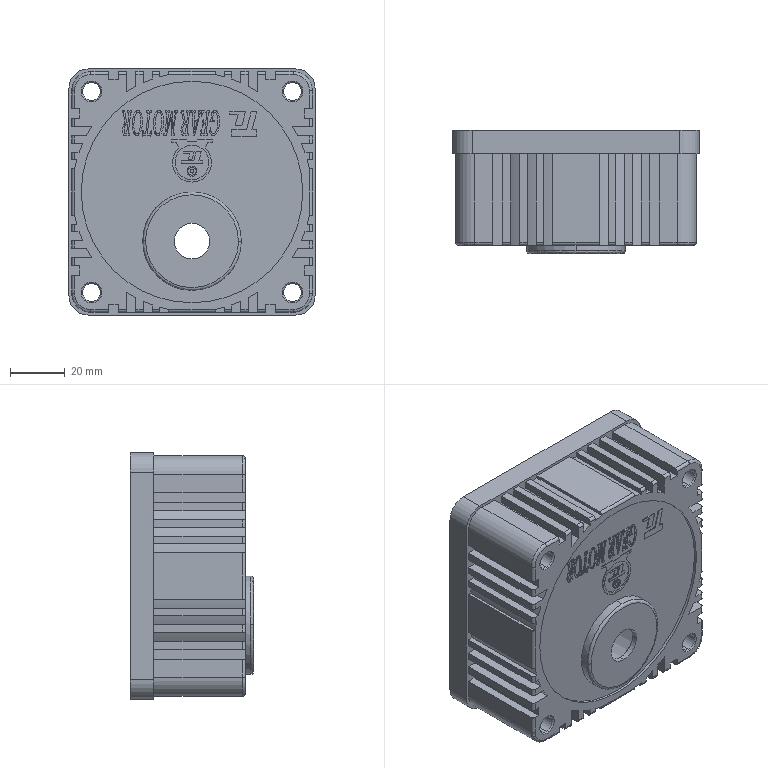Part | STEP file | 1 solid | 850 faces | box 90 x 45 x 90 mm | volume 121396 mm3 | plane 392 | spline 285 | cylinder 153 | cone 20 | commonest cylinder face diameters 2 x36 87.5 x24 3.3 x8 6.5 x8 11 x8 14 x8